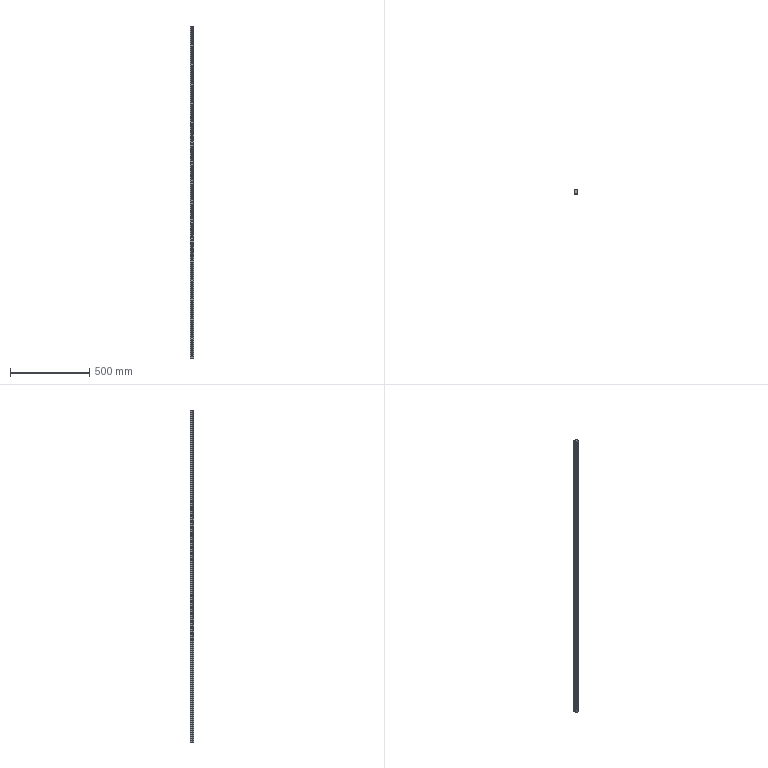Part | NX | features BREP 1 | 1 solid | 319 faces | box 23 x 22 x 2100 mm | volume 864462 mm3 | plane 171 | cylinder 148 | commonest cylinder face diameters 7 x70 11 x70 2 x4 4.6 x4